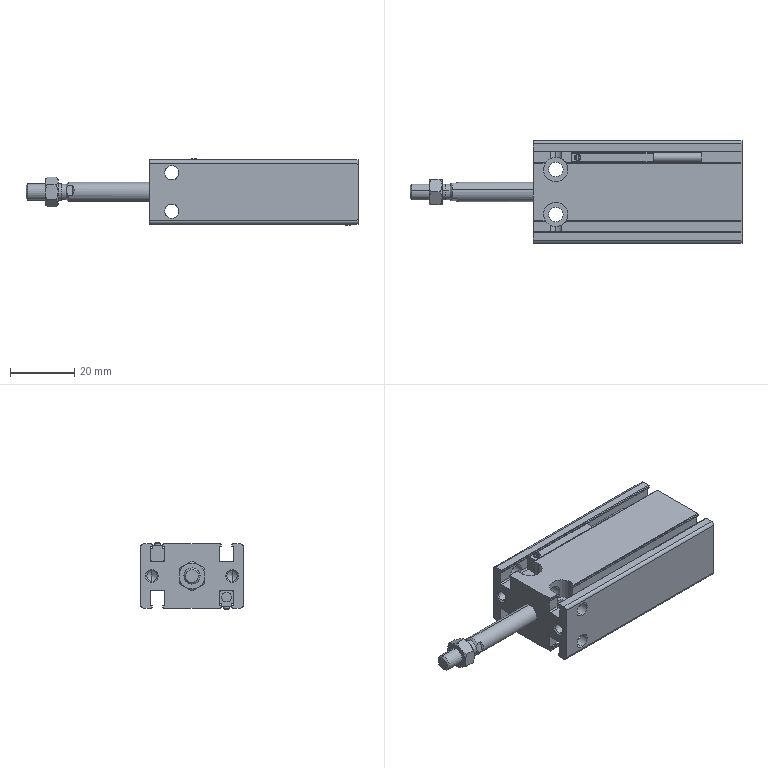Part | SolidWorks | 5 solids | 294 faces | box 103.415 x 32 x 20.8 mm | volume 30236 mm3 | cylinder 128 | plane 113 | cone 53 | commonest cylinder face diameters 0.4 x40 0.8 x16 4.5 x16 2 x8 3.242 x8 7.6 x8